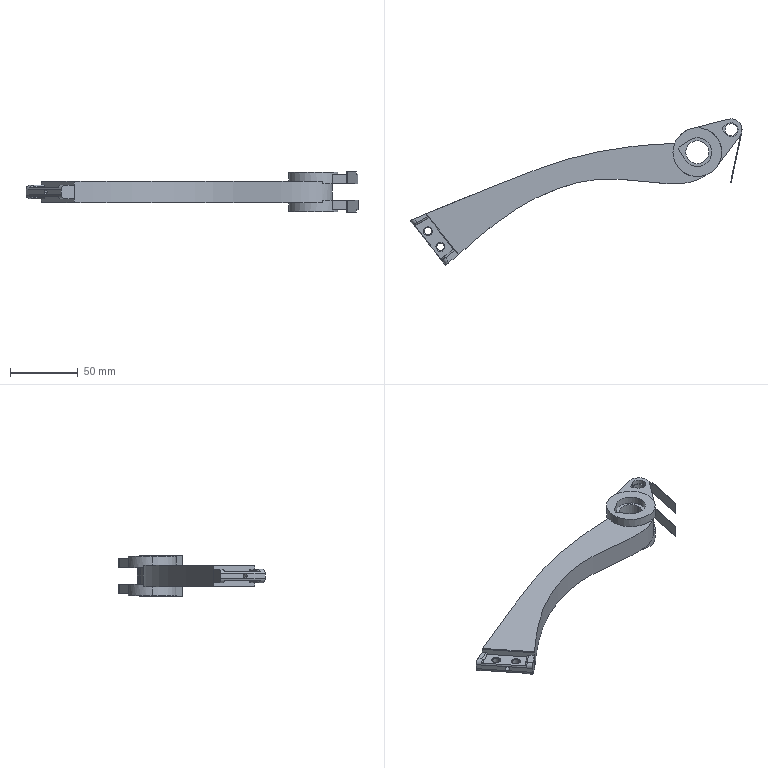Part | SolidWorks | features ICE 18, Fillet 5, Extrusion 1, MirrorPattern 1 | 1 solid | 114 faces | box 245.132 x 107.958 x 30 mm | volume 99502 mm3 | plane 60 | cylinder 39 | torus 10 | spline 5 | commonest cylinder face diameters 16 x5 2.4 x4 5.6 x4 9 x4 36 x4 10.3 x3